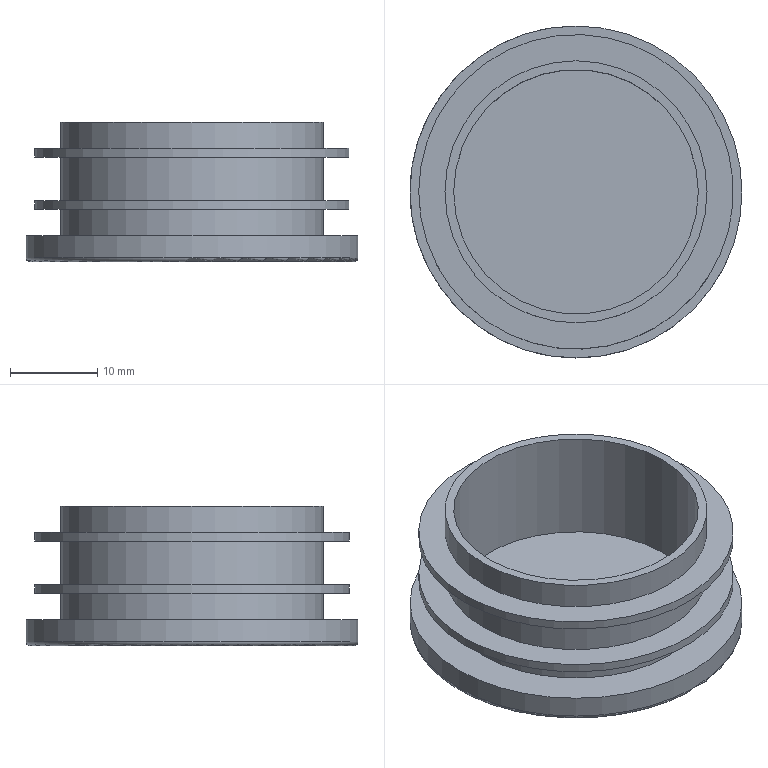Part | STEP file | 7101208W | 1 solid | 16 faces | box 38 x 38 x 16 mm | volume 5202 mm3 | plane 8 | cylinder 7 | torus 1 | commonest cylinder face diameters 30 x3 36 x2 28 x1 38 x1
STEP:
#1=CARTESIAN_POINT('',(0.,0.,0.));
#2=DIRECTION('',(0.,0.,1.));
#3=DIRECTION('',(1.,0.,0.));
#4=AXIS2_PLACEMENT_3D('',#1,#2,#3);
#5=CARTESIAN_POINT('',(15.,0.,3.));
#6=VERTEX_POINT('',#5);
#7=CARTESIAN_POINT('',(-15.,0.,3.));
#8=VERTEX_POINT('',#7);
#9=CARTESIAN_POINT('',(0.,0.,3.));
#10=DIRECTION('',(0.,0.,1.));
#11=DIRECTION('',(1.,0.,0.));
#12=AXIS2_PLACEMENT_3D('',#9,#10,#11);
#13=CIRCLE('',#12,15.);
#14=CARTESIAN_POINT('',(0.,0.,3.));
#15=DIRECTION('',(0.,0.,1.));
#16=DIRECTION('',(1.,0.,0.));
#17=AXIS2_PLACEMENT_3D('',#14,#15,#16);
#18=PLANE('',#17);
#19=CARTESIAN_POINT('',(0.,0.));
#20=DIRECTION('',(1.,0.));
#21=AXIS2_PLACEMENT_2D('',#19,#20);
#22=CIRCLE('',#21,15.);
#23=(GEOMETRIC_REPRESENTATION_CONTEXT(2)PARAMETRIC_REPRESENTATION_CONTEXT()REPRESENTATION_CONTEXT('',''));
#24=DEFINITIONAL_REPRESENTATION('',(#22),#23);
#25=PCURVE('',#18,#24);
#26=CARTESIAN_POINT('',(0.,0.,3.));
#27=DIRECTION('',(0.,0.,-1.));
#28=DIRECTION('',(-1.,0.,0.));
#29=AXIS2_PLACEMENT_3D('',#26,#27,#28);
#30=CYLINDRICAL_SURFACE('',#29,15.);
#31=CARTESIAN_POINT('',(3.142,0.));
#32=DIRECTION('',(-1.,0.));
#33=VECTOR('',#32,1.);
#34=LINE('',#31,#33);
#35=(GEOMETRIC_REPRESENTATION_CONTEXT(2)PARAMETRIC_REPRESENTATION_CONTEXT()REPRESENTATION_CONTEXT('',''));
#36=DEFINITIONAL_REPRESENTATION('',(#34),#35);
#37=PCURVE('',#30,#36);
#38=SURFACE_CURVE('',#13,(#25,#37),.PCURVE_S1.);
#39=EDGE_CURVE('',#6,#8,#38,.T.);
#40=ORIENTED_EDGE('',*,*,#39,.F.);
#41=CARTESIAN_POINT('',(0.,0.,3.));
#42=DIRECTION('',(0.,0.,1.));
#43=DIRECTION('',(1.,0.,0.));
#44=AXIS2_PLACEMENT_3D('',#41,#42,#43);
#45=CIRCLE('',#44,15.);
#46=CARTESIAN_POINT('',(0.,0.));
#47=DIRECTION('',(1.,0.));
#48=AXIS2_PLACEMENT_2D('',#46,#47);
#49=CIRCLE('',#48,15.);
#50=(GEOMETRIC_REPRESENTATION_CONTEXT(2)PARAMETRIC_REPRESENTATION_CONTEXT()REPRESENTATION_CONTEXT('',''));
#51=DEFINITIONAL_REPRESENTATION('',(#49),#50);
#52=PCURVE('',#18,#51);
#53=CARTESIAN_POINT('',(9.425,0.));
#54=DIRECTION('',(-1.,0.));
#55=VECTOR('',#54,1.);
#56=LINE('',#53,#55);
#57=(GEOMETRIC_REPRESENTATION_CONTEXT(2)PARAMETRIC_REPRESENTATION_CONTEXT()REPRESENTATION_CONTEXT('',''));
#58=DEFINITIONAL_REPRESENTATION('',(#56),#57);
#59=PCURVE('',#30,#58);
#60=SURFACE_CURVE('',#45,(#52,#59),.PCURVE_S1.);
#61=EDGE_CURVE('',#8,#6,#60,.T.);
#62=ORIENTED_EDGE('',*,*,#61,.F.);
#63=EDGE_LOOP('',(#40,#62));
#64=FACE_BOUND('',#63,.T.);
#65=CARTESIAN_POINT('',(19.,0.,3.));
#66=VERTEX_POINT('',#65);
#67=CARTESIAN_POINT('',(0.,0.,3.));
#68=DIRECTION('',(0.,0.,1.));
#69=DIRECTION('',(1.,0.,0.));
#70=AXIS2_PLACEMENT_3D('',#67,#68,#69);
#71=CIRCLE('',#70,19.);
#72=CARTESIAN_POINT('',(0.,0.));
#73=DIRECTION('',(1.,0.));
#74=AXIS2_PLACEMENT_2D('',#72,#73);
#75=CIRCLE('',#74,19.);
#76=(GEOMETRIC_REPRESENTATION_CONTEXT(2)PARAMETRIC_REPRESENTATION_CONTEXT()REPRESENTATION_CONTEXT('',''));
#77=DEFINITIONAL_REPRESENTATION('',(#75),#76);
#78=PCURVE('',#18,#77);
#79=CARTESIAN_POINT('',(0.,0.,3.));
#80=DIRECTION('',(0.,0.,-1.));
#81=DIRECTION('',(-1.,0.,0.));
#82=AXIS2_PLACEMENT_3D('',#79,#80,#81);
#83=CYLINDRICAL_SURFACE('',#82,19.);
#84=CARTESIAN_POINT('',(9.425,0.));
#85=DIRECTION('',(-1.,0.));
#86=VECTOR('',#85,1.);
#87=LINE('',#84,#86);
#88=(GEOMETRIC_REPRESENTATION_CONTEXT(2)PARAMETRIC_REPRESENTATION_CONTEXT()REPRESENTATION_CONTEXT('',''));
#89=DEFINITIONAL_REPRESENTATION('',(#87),#88);
#90=PCURVE('',#83,#89);
#91=SURFACE_CURVE('',#71,(#78,#90),.PCURVE_S1.);
#92=EDGE_CURVE('',#66,#66,#91,.T.);
#93=ORIENTED_EDGE('',*,*,#92,.T.);
#94=EDGE_LOOP('',(#93));
#95=FACE_BOUND('',#94,.T.);
#96=ADVANCED_FACE('',(#64,#95),#18,.T.);
#97=CARTESIAN_POINT('',(19.,0.,0.5));
#98=VERTEX_POINT('',#97);
#99=CARTESIAN_POINT('',(0.,0.,0.5));
#100=DIRECTION('',(0.,0.,1.));
#101=DIRECTION('',(1.,0.,0.));
#102=AXIS2_PLACEMENT_3D('',#99,#100,#101);
#103=CIRCLE('',#102,19.);
#104=CARTESIAN_POINT('',(9.425,2.5));
#105=DIRECTION('',(-1.,0.));
#106=VECTOR('',#105,1.);
#107=LINE('',#104,#106);
#108=(GEOMETRIC_REPRESENTATION_CONTEXT(2)PARAMETRIC_REPRESENTATION_CONTEXT()REPRESENTATION_CONTEXT('',''));
#109=DEFINITIONAL_REPRESENTATION('',(#107),#108);
#110=PCURVE('',#83,#109);
#111=CARTESIAN_POINT('',(0.,0.,0.5));
#112=DIRECTION('',(0.,0.,1.));
#113=DIRECTION('',(1.,0.,0.));
#114=AXIS2_PLACEMENT_3D('',#111,#112,#113);
#115=TOROIDAL_SURFACE('',#114,18.5,0.5);
#116=CARTESIAN_POINT('',(0.,6.283));
#117=DIRECTION('',(1.,0.));
#118=VECTOR('',#117,1.);
#119=LINE('',#116,#118);
#120=(GEOMETRIC_REPRESENTATION_CONTEXT(2)PARAMETRIC_REPRESENTATION_CONTEXT()REPRESENTATION_CONTEXT('',''));
#121=DEFINITIONAL_REPRESENTATION('',(#119),#120);
#122=PCURVE('',#115,#121);
#123=SURFACE_CURVE('',#103,(#110,#122),.PCURVE_S1.);
#124=EDGE_CURVE('',#98,#98,#123,.T.);
#125=ORIENTED_EDGE('',*,*,#124,.T.);
#126=CARTESIAN_POINT('',(19.,0.,3.));
#127=CARTESIAN_POINT('',(19.,0.,0.5));
#128=B_SPLINE_CURVE_WITH_KNOTS('',1,(#126,#127),.UNSPECIFIED.,.F.,.F.,(2,2),(0.,2.5),.PIECEWISE_BEZIER_KNOTS.);
#129=CARTESIAN_POINT('',(3.142,0.));
#130=DIRECTION('',(0.,1.));
#131=VECTOR('',#130,1.);
#132=LINE('',#129,#131);
#133=(GEOMETRIC_REPRESENTATION_CONTEXT(2)PARAMETRIC_REPRESENTATION_CONTEXT()REPRESENTATION_CONTEXT('',''));
#134=DEFINITIONAL_REPRESENTATION('',(#132),#133);
#135=PCURVE('',#83,#134);
#136=CARTESIAN_POINT('',(9.425,0.));
#137=DIRECTION('',(0.,1.));
#138=VECTOR('',#137,1.);
#139=LINE('',#136,#138);
#140=(GEOMETRIC_REPRESENTATION_CONTEXT(2)PARAMETRIC_REPRESENTATION_CONTEXT()REPRESENTATION_CONTEXT('',''));
#141=DEFINITIONAL_REPRESENTATION('',(#139),#140);
#142=PCURVE('',#83,#141);
#143=SEAM_CURVE('',#128,(#135,#142),.PCURVE_S1.);
#144=EDGE_CURVE('',#66,#98,#143,.T.);
#145=ORIENTED_EDGE('',*,*,#144,.F.);
#146=ORIENTED_EDGE('',*,*,#92,.F.);
#147=ORIENTED_EDGE('',*,*,#144,.T.);
#148=EDGE_LOOP('',(#125,#145,#146,#147));
#149=FACE_BOUND('',#148,.T.);
#150=ADVANCED_FACE('',(#149),#83,.T.);
#151=CARTESIAN_POINT('',(18.5,0.,0.));
#152=VERTEX_POINT('',#151);
#153=CARTESIAN_POINT('',(0.,0.,0.));
#154=DIRECTION('',(0.,0.,-1.));
#155=DIRECTION('',(1.,0.,0.));
#156=AXIS2_PLACEMENT_3D('',#153,#154,#155);
#157=CIRCLE('',#156,18.5);
#158=CARTESIAN_POINT('',(0.,0.,0.));
#159=DIRECTION('',(0.,0.,1.));
#160=DIRECTION('',(1.,0.,0.));
#161=AXIS2_PLACEMENT_3D('',#158,#159,#160);
#162=PLANE('',#161);
#163=CARTESIAN_POINT('',(18.5,0.));
#164=CARTESIAN_POINT('',(18.5,-32.043));
#165=CARTESIAN_POINT('',(-9.25,-16.021));
#166=CARTESIAN_POINT('',(-37.,0.));
#167=CARTESIAN_POINT('',(-9.25,16.021));
#168=CARTESIAN_POINT('',(18.5,32.043));
#169=CARTESIAN_POINT('',(18.5,0.));
#170=(BOUNDED_CURVE()B_SPLINE_CURVE(2,(#163,#164,#165,#166,#167,#168,#169),.UNSPECIFIED.,.T.,.F.)B_SPLINE_CURVE_WITH_KNOTS((1,2,2,2,2,1),(-2.094,0.,2.094,4.189,6.283,8.378),.UNSPECIFIED.)CURVE()GEOMETRIC_REPRESENTATION_ITEM()RATIONAL_B_SPLINE_CURVE((1.,0.5,1.,0.5,1.,0.5,1.))REPRESENTATION_ITEM(''));
#171=(GEOMETRIC_REPRESENTATION_CONTEXT(2)PARAMETRIC_REPRESENTATION_CONTEXT()REPRESENTATION_CONTEXT('',''));
#172=DEFINITIONAL_REPRESENTATION('',(#170),#171);
#173=PCURVE('',#162,#172);
#174=CARTESIAN_POINT('',(6.283,4.712));
#175=DIRECTION('',(-1.,0.));
#176=VECTOR('',#175,1.);
#177=LINE('',#174,#176);
#178=(GEOMETRIC_REPRESENTATION_CONTEXT(2)PARAMETRIC_REPRESENTATION_CONTEXT()REPRESENTATION_CONTEXT('',''));
#179=DEFINITIONAL_REPRESENTATION('',(#177),#178);
#180=PCURVE('',#115,#179);
#181=SURFACE_CURVE('',#157,(#173,#180),.PCURVE_S1.);
#182=EDGE_CURVE('',#152,#152,#181,.T.);
#183=ORIENTED_EDGE('',*,*,#182,.T.);
#184=EDGE_LOOP('',(#183));
#185=FACE_BOUND('',#184,.T.);
#186=ADVANCED_FACE('',(#185),#162,.F.);
#187=CARTESIAN_POINT('',(-15.,0.,6.));
#188=VERTEX_POINT('',#187);
#189=CARTESIAN_POINT('',(0.,0.,6.));
#190=DIRECTION('',(0.,0.,-1.));
#191=DIRECTION('',(-1.,0.,0.));
#192=AXIS2_PLACEMENT_3D('',#189,#190,#191);
#193=CIRCLE('',#192,15.);
#194=CARTESIAN_POINT('',(0.,-3.));
#195=DIRECTION('',(1.,0.));
#196=VECTOR('',#195,1.);
#197=LINE('',#194,#196);
#198=(GEOMETRIC_REPRESENTATION_CONTEXT(2)PARAMETRIC_REPRESENTATION_CONTEXT()REPRESENTATION_CONTEXT('',''));
#199=DEFINITIONAL_REPRESENTATION('',(#197),#198);
#200=PCURVE('',#30,#199);
#201=CARTESIAN_POINT('',(-15.,0.,6.));
#202=DIRECTION('',(0.,0.,-1.));
#203=DIRECTION('',(-1.,0.,0.));
#204=AXIS2_PLACEMENT_3D('',#201,#202,#203);
#205=PLANE('',#204);
#206=CARTESIAN_POINT('',(-15.,0.));
#207=DIRECTION('',(1.,0.));
#208=AXIS2_PLACEMENT_2D('',#206,#207);
#209=CIRCLE('',#208,15.);
#210=(GEOMETRIC_REPRESENTATION_CONTEXT(2)PARAMETRIC_REPRESENTATION_CONTEXT()REPRESENTATION_CONTEXT('',''));
#211=DEFINITIONAL_REPRESENTATION('',(#209),#210);
#212=PCURVE('',#205,#211);
#213=SURFACE_CURVE('',#193,(#200,#212),.PCURVE_S1.);
#214=EDGE_CURVE('',#188,#188,#213,.T.);
#215=ORIENTED_EDGE('',*,*,#214,.T.);
#216=CARTESIAN_POINT('',(-15.,0.,6.));
#217=CARTESIAN_POINT('',(-15.,0.,3.));
#218=B_SPLINE_CURVE_WITH_KNOTS('',1,(#216,#217),.UNSPECIFIED.,.F.,.F.,(2,2),(-3.,0.),.PIECEWISE_BEZIER_KNOTS.);
#219=CARTESIAN_POINT('',(6.283,0.));
#220=DIRECTION('',(0.,1.));
#221=VECTOR('',#220,1.);
#222=LINE('',#219,#221);
#223=(GEOMETRIC_REPRESENTATION_CONTEXT(2)PARAMETRIC_REPRESENTATION_CONTEXT()REPRESENTATION_CONTEXT('',''));
#224=DEFINITIONAL_REPRESENTATION('',(#222),#223);
#225=PCURVE('',#30,#224);
#226=CARTESIAN_POINT('',(0.,0.));
#227=DIRECTION('',(0.,1.));
#228=VECTOR('',#227,1.);
#229=LINE('',#226,#228);
#230=(GEOMETRIC_REPRESENTATION_CONTEXT(2)PARAMETRIC_REPRESENTATION_CONTEXT()REPRESENTATION_CONTEXT('',''));
#231=DEFINITIONAL_REPRESENTATION('',(#229),#230);
#232=PCURVE('',#30,#231);
#233=SEAM_CURVE('',#218,(#225,#232),.PCURVE_S1.);
#234=EDGE_CURVE('',#188,#8,#233,.T.);
#235=ORIENTED_EDGE('',*,*,#234,.T.);
#236=ORIENTED_EDGE('',*,*,#61,.T.);
#237=ORIENTED_EDGE('',*,*,#39,.T.);
#238=ORIENTED_EDGE('',*,*,#234,.F.);
#239=EDGE_LOOP('',(#215,#235,#236,#237,#238));
#240=FACE_BOUND('',#239,.T.);
#241=ADVANCED_FACE('',(#240),#30,.T.);
#242=CARTESIAN_POINT('',(-18.,0.,6.));
#243=VERTEX_POINT('',#242);
#244=CARTESIAN_POINT('',(0.,0.,6.));
#245=DIRECTION('',(0.,0.,-1.));
#246=DIRECTION('',(-1.,0.,0.));
#247=AXIS2_PLACEMENT_3D('',#244,#245,#246);
#248=CIRCLE('',#247,18.);
#249=CARTESIAN_POINT('',(-15.,0.));
#250=DIRECTION('',(1.,0.));
#251=AXIS2_PLACEMENT_2D('',#249,#250);
#252=CIRCLE('',#251,18.);
#253=(GEOMETRIC_REPRESENTATION_CONTEXT(2)PARAMETRIC_REPRESENTATION_CONTEXT()REPRESENTATION_CONTEXT('',''));
#254=DEFINITIONAL_REPRESENTATION('',(#252),#253);
#255=PCURVE('',#205,#254);
#256=CARTESIAN_POINT('',(0.,0.,3.));
#257=DIRECTION('',(0.,0.,-1.));
#258=DIRECTION('',(-1.,0.,0.));
#259=AXIS2_PLACEMENT_3D('',#256,#257,#258);
#260=CYLINDRICAL_SURFACE('',#259,18.);
#261=CARTESIAN_POINT('',(0.,-3.));
#262=DIRECTION('',(1.,0.));
#263=VECTOR('',#262,1.);
#264=LINE('',#261,#263);
#265=(GEOMETRIC_REPRESENTATION_CONTEXT(2)PARAMETRIC_REPRESENTATION_CONTEXT()REPRESENTATION_CONTEXT('',''));
#266=DEFINITIONAL_REPRESENTATION('',(#264),#265);
#267=PCURVE('',#260,#266);
#268=SURFACE_CURVE('',#248,(#255,#267),.PCURVE_S1.);
#269=EDGE_CURVE('',#243,#243,#268,.T.);
#270=ORIENTED_EDGE('',*,*,#269,.T.);
#271=EDGE_LOOP('',(#270));
#272=FACE_BOUND('',#271,.T.);
#273=ORIENTED_EDGE('',*,*,#214,.F.);
#274=EDGE_LOOP('',(#273));
#275=FACE_BOUND('',#274,.T.);
#276=ADVANCED_FACE('',(#272,#275),#205,.T.);
#277=CARTESIAN_POINT('',(-18.,0.,7.));
#278=VERTEX_POINT('',#277);
#279=CARTESIAN_POINT('',(0.,0.,7.));
#280=DIRECTION('',(0.,0.,-1.));
#281=DIRECTION('',(-1.,0.,0.));
#282=AXIS2_PLACEMENT_3D('',#279,#280,#281);
#283=CIRCLE('',#282,18.);
#284=CARTESIAN_POINT('',(0.,-4.));
#285=DIRECTION('',(1.,0.));
#286=VECTOR('',#285,1.);
#287=LINE('',#284,#286);
#288=(GEOMETRIC_REPRESENTATION_CONTEXT(2)PARAMETRIC_REPRESENTATION_CONTEXT()REPRESENTATION_CONTEXT('',''));
#289=DEFINITIONAL_REPRESENTATION('',(#287),#288);
#290=PCURVE('',#260,#289);
#291=CARTESIAN_POINT('',(-18.,0.,7.));
#292=DIRECTION('',(0.,0.,1.));
#293=DIRECTION('',(1.,0.,0.));
#294=AXIS2_PLACEMENT_3D('',#291,#292,#293);
#295=PLANE('',#294);
#296=CARTESIAN_POINT('',(0.,0.));
#297=CARTESIAN_POINT('',(0.,31.177));
#298=CARTESIAN_POINT('',(27.,15.588));
#299=CARTESIAN_POINT('',(54.,0.));
#300=CARTESIAN_POINT('',(27.,-15.588));
#301=CARTESIAN_POINT('',(0.,-31.177));
#302=CARTESIAN_POINT('',(0.,0.));
#303=(BOUNDED_CURVE()B_SPLINE_CURVE(2,(#296,#297,#298,#299,#300,#301,#302),.UNSPECIFIED.,.T.,.F.)B_SPLINE_CURVE_WITH_KNOTS((1,2,2,2,2,1),(-2.094,0.,2.094,4.189,6.283,8.378),.UNSPECIFIED.)CURVE()GEOMETRIC_REPRESENTATION_ITEM()RATIONAL_B_SPLINE_CURVE((1.,0.5,1.,0.5,1.,0.5,1.))REPRESENTATION_ITEM(''));
#304=(GEOMETRIC_REPRESENTATION_CONTEXT(2)PARAMETRIC_REPRESENTATION_CONTEXT()REPRESENTATION_CONTEXT('',''));
#305=DEFINITIONAL_REPRESENTATION('',(#303),#304);
#306=PCURVE('',#295,#305);
#307=SURFACE_CURVE('',#283,(#290,#306),.PCURVE_S1.);
#308=EDGE_CURVE('',#278,#278,#307,.T.);
#309=ORIENTED_EDGE('',*,*,#308,.T.);
#310=CARTESIAN_POINT('',(-18.,0.,7.));
#311=CARTESIAN_POINT('',(-18.,0.,6.));
#312=B_SPLINE_CURVE_WITH_KNOTS('',1,(#310,#311),.UNSPECIFIED.,.F.,.F.,(2,2),(-4.,-3.),.PIECEWISE_BEZIER_KNOTS.);
#313=CARTESIAN_POINT('',(6.283,0.));
#314=DIRECTION('',(0.,1.));
#315=VECTOR('',#314,1.);
#316=LINE('',#313,#315);
#317=(GEOMETRIC_REPRESENTATION_CONTEXT(2)PARAMETRIC_REPRESENTATION_CONTEXT()REPRESENTATION_CONTEXT('',''));
#318=DEFINITIONAL_REPRESENTATION('',(#316),#317);
#319=PCURVE('',#260,#318);
#320=CARTESIAN_POINT('',(0.,0.));
#321=DIRECTION('',(0.,1.));
#322=VECTOR('',#321,1.);
#323=LINE('',#320,#322);
#324=(GEOMETRIC_REPRESENTATION_CONTEXT(2)PARAMETRIC_REPRESENTATION_CONTEXT()REPRESENTATION_CONTEXT('',''));
#325=DEFINITIONAL_REPRESENTATION('',(#323),#324);
#326=PCURVE('',#260,#325);
#327=SEAM_CURVE('',#312,(#319,#326),.PCURVE_S1.);
#328=EDGE_CURVE('',#278,#243,#327,.T.);
#329=ORIENTED_EDGE('',*,*,#328,.T.);
#330=ORIENTED_EDGE('',*,*,#269,.F.);
#331=ORIENTED_EDGE('',*,*,#328,.F.);
#332=EDGE_LOOP('',(#309,#329,#330,#331));
#333=FACE_BOUND('',#332,.T.);
#334=ADVANCED_FACE('',(#333),#260,.T.);
#335=CARTESIAN_POINT('',(-15.,0.,7.));
#336=VERTEX_POINT('',#335);
#337=CARTESIAN_POINT('',(0.,0.,7.));
#338=DIRECTION('',(0.,0.,-1.));
#339=DIRECTION('',(-1.,0.,0.));
#340=AXIS2_PLACEMENT_3D('',#337,#338,#339);
#341=CIRCLE('',#340,15.);
#342=CARTESIAN_POINT('',(3.,0.));
#343=CARTESIAN_POINT('',(3.,25.981));
#344=CARTESIAN_POINT('',(25.5,12.99));
#345=CARTESIAN_POINT('',(48.,0.));
#346=CARTESIAN_POINT('',(25.5,-12.99));
#347=CARTESIAN_POINT('',(3.,-25.981));
#348=CARTESIAN_POINT('',(3.,0.));
#349=(BOUNDED_CURVE()B_SPLINE_CURVE(2,(#342,#343,#344,#345,#346,#347,#348),.UNSPECIFIED.,.T.,.F.)B_SPLINE_CURVE_WITH_KNOTS((1,2,2,2,2,1),(-2.094,0.,2.094,4.189,6.283,8.378),.UNSPECIFIED.)CURVE()GEOMETRIC_REPRESENTATION_ITEM()RATIONAL_B_SPLINE_CURVE((1.,0.5,1.,0.5,1.,0.5,1.))REPRESENTATION_ITEM(''));
#350=(GEOMETRIC_REPRESENTATION_CONTEXT(2)PARAMETRIC_REPRESENTATION_CONTEXT()REPRESENTATION_CONTEXT('',''));
#351=DEFINITIONAL_REPRESENTATION('',(#349),#350);
#352=PCURVE('',#295,#351);
#353=CARTESIAN_POINT('',(0.,0.,3.));
#354=DIRECTION('',(0.,0.,-1.));
#355=DIRECTION('',(-1.,0.,0.));
#356=AXIS2_PLACEMENT_3D('',#353,#354,#355);
#357=CYLINDRICAL_SURFACE('',#356,15.);
#358=CARTESIAN_POINT('',(0.,-4.));
#359=DIRECTION('',(1.,0.));
#360=VECTOR('',#359,1.);
#361=LINE('',#358,#360);
#362=(GEOMETRIC_REPRESENTATION_CONTEXT(2)PARAMETRIC_REPRESENTATION_CONTEXT()REPRESENTATION_CONTEXT('',''));
#363=DEFINITIONAL_REPRESENTATION('',(#361),#362);
#364=PCURVE('',#357,#363);
#365=SURFACE_CURVE('',#341,(#352,#364),.PCURVE_S1.);
#366=EDGE_CURVE('',#336,#336,#365,.T.);
#367=ORIENTED_EDGE('',*,*,#366,.T.);
#368=EDGE_LOOP('',(#367));
#369=FACE_BOUND('',#368,.T.);
#370=ORIENTED_EDGE('',*,*,#308,.F.);
#371=EDGE_LOOP('',(#370));
#372=FACE_BOUND('',#371,.T.);
#373=ADVANCED_FACE('',(#369,#372),#295,.T.);
#374=CARTESIAN_POINT('',(-15.,0.,12.));
#375=VERTEX_POINT('',#374);
#376=CARTESIAN_POINT('',(0.,0.,12.));
#377=DIRECTION('',(0.,0.,-1.));
#378=DIRECTION('',(-1.,0.,0.));
#379=AXIS2_PLACEMENT_3D('',#376,#377,#378);
#380=CIRCLE('',#379,15.);
#381=CARTESIAN_POINT('',(0.,-9.));
#382=DIRECTION('',(1.,0.));
#383=VECTOR('',#382,1.);
#384=LINE('',#381,#383);
#385=(GEOMETRIC_REPRESENTATION_CONTEXT(2)PARAMETRIC_REPRESENTATION_CONTEXT()REPRESENTATION_CONTEXT('',''));
#386=DEFINITIONAL_REPRESENTATION('',(#384),#385);
#387=PCURVE('',#357,#386);
#388=CARTESIAN_POINT('',(-15.,0.,12.));
#389=DIRECTION('',(0.,0.,-1.));
#390=DIRECTION('',(-1.,0.,0.));
#391=AXIS2_PLACEMENT_3D('',#388,#389,#390);
#392=PLANE('',#391);
#393=CARTESIAN_POINT('',(-15.,0.));
#394=DIRECTION('',(1.,0.));
#395=AXIS2_PLACEMENT_2D('',#393,#394);
#396=CIRCLE('',#395,15.);
#397=(GEOMETRIC_REPRESENTATION_CONTEXT(2)PARAMETRIC_REPRESENTATION_CONTEXT()REPRESENTATION_CONTEXT('',''));
#398=DEFINITIONAL_REPRESENTATION('',(#396),#397);
#399=PCURVE('',#392,#398);
#400=SURFACE_CURVE('',#380,(#387,#399),.PCURVE_S1.);
#401=EDGE_CURVE('',#375,#375,#400,.T.);
#402=ORIENTED_EDGE('',*,*,#401,.T.);
#403=CARTESIAN_POINT('',(-15.,0.,12.));
#404=CARTESIAN_POINT('',(-15.,0.,7.));
#405=B_SPLINE_CURVE_WITH_KNOTS('',1,(#403,#404),.UNSPECIFIED.,.F.,.F.,(2,2),(-9.,-4.),.PIECEWISE_BEZIER_KNOTS.);
#406=CARTESIAN_POINT('',(6.283,0.));
#407=DIRECTION('',(0.,1.));
#408=VECTOR('',#407,1.);
#409=LINE('',#406,#408);
#410=(GEOMETRIC_REPRESENTATION_CONTEXT(2)PARAMETRIC_REPRESENTATION_CONTEXT()REPRESENTATION_CONTEXT('',''));
#411=DEFINITIONAL_REPRESENTATION('',(#409),#410);
#412=PCURVE('',#357,#411);
#413=CARTESIAN_POINT('',(0.,0.));
#414=DIRECTION('',(0.,1.));
#415=VECTOR('',#414,1.);
#416=LINE('',#413,#415);
#417=(GEOMETRIC_REPRESENTATION_CONTEXT(2)PARAMETRIC_REPRESENTATION_CONTEXT()REPRESENTATION_CONTEXT('',''));
#418=DEFINITIONAL_REPRESENTATION('',(#416),#417);
#419=PCURVE('',#357,#418);
#420=SEAM_CURVE('',#405,(#412,#419),.PCURVE_S1.);
#421=EDGE_CURVE('',#375,#336,#420,.T.);
#422=ORIENTED_EDGE('',*,*,#421,.T.);
#423=ORIENTED_EDGE('',*,*,#366,.F.);
#424=ORIENTED_EDGE('',*,*,#421,.F.);
#425=EDGE_LOOP('',(#402,#422,#423,#424));
#426=FACE_BOUND('',#425,.T.);
#427=ADVANCED_FACE('',(#426),#357,.T.);
#428=CARTESIAN_POINT('',(-18.,0.,12.));
#429=VERTEX_POINT('',#428);
#430=CARTESIAN_POINT('',(0.,0.,12.));
#431=DIRECTION('',(0.,0.,-1.));
#432=DIRECTION('',(-1.,0.,0.));
#433=AXIS2_PLACEMENT_3D('',#430,#431,#432);
#434=CIRCLE('',#433,18.);
#435=CARTESIAN_POINT('',(-15.,0.));
#436=DIRECTION('',(1.,0.));
#437=AXIS2_PLACEMENT_2D('',#435,#436);
#438=CIRCLE('',#437,18.);
#439=(GEOMETRIC_REPRESENTATION_CONTEXT(2)PARAMETRIC_REPRESENTATION_CONTEXT()REPRESENTATION_CONTEXT('',''));
#440=DEFINITIONAL_REPRESENTATION('',(#438),#439);
#441=PCURVE('',#392,#440);
#442=CARTESIAN_POINT('',(0.,0.,3.));
#443=DIRECTION('',(0.,0.,-1.));
#444=DIRECTION('',(-1.,0.,0.));
#445=AXIS2_PLACEMENT_3D('',#442,#443,#444);
#446=CYLINDRICAL_SURFACE('',#445,18.);
#447=CARTESIAN_POINT('',(0.,-9.));
#448=DIRECTION('',(1.,0.));
#449=VECTOR('',#448,1.);
#450=LINE('',#447,#449);
#451=(GEOMETRIC_REPRESENTATION_CONTEXT(2)PARAMETRIC_REPRESENTATION_CONTEXT()REPRESENTATION_CONTEXT('',''));
#452=DEFINITIONAL_REPRESENTATION('',(#450),#451);
#453=PCURVE('',#446,#452);
#454=SURFACE_CURVE('',#434,(#441,#453),.PCURVE_S1.);
#455=EDGE_CURVE('',#429,#429,#454,.T.);
#456=ORIENTED_EDGE('',*,*,#455,.T.);
#457=EDGE_LOOP('',(#456));
#458=FACE_BOUND('',#457,.T.);
#459=ORIENTED_EDGE('',*,*,#401,.F.);
#460=EDGE_LOOP('',(#459));
#461=FACE_BOUND('',#460,.T.);
#462=ADVANCED_FACE('',(#458,#461),#392,.T.);
#463=CARTESIAN_POINT('',(-18.,0.,13.));
#464=VERTEX_POINT('',#463);
#465=CARTESIAN_POINT('',(0.,0.,13.));
#466=DIRECTION('',(0.,0.,-1.));
#467=DIRECTION('',(-1.,0.,0.));
#468=AXIS2_PLACEMENT_3D('',#465,#466,#467);
#469=CIRCLE('',#468,18.);
#470=CARTESIAN_POINT('',(0.,-10.));
#471=DIRECTION('',(1.,0.));
#472=VECTOR('',#471,1.);
#473=LINE('',#470,#472);
#474=(GEOMETRIC_REPRESENTATION_CONTEXT(2)PARAMETRIC_REPRESENTATION_CONTEXT()REPRESENTATION_CONTEXT('',''));
#475=DEFINITIONAL_REPRESENTATION('',(#473),#474);
#476=PCURVE('',#446,#475);
#477=CARTESIAN_POINT('',(-18.,0.,13.));
#478=DIRECTION('',(0.,0.,1.));
#479=DIRECTION('',(1.,0.,0.));
#480=AXIS2_PLACEMENT_3D('',#477,#478,#479);
#481=PLANE('',#480);
#482=CARTESIAN_POINT('',(0.,0.));
#483=CARTESIAN_POINT('',(0.,31.177));
#484=CARTESIAN_POINT('',(27.,15.588));
#485=CARTESIAN_POINT('',(54.,0.));
#486=CARTESIAN_POINT('',(27.,-15.588));
#487=CARTESIAN_POINT('',(0.,-31.177));
#488=CARTESIAN_POINT('',(0.,0.));
#489=(BOUNDED_CURVE()B_SPLINE_CURVE(2,(#482,#483,#484,#485,#486,#487,#488),.UNSPECIFIED.,.T.,.F.)B_SPLINE_CURVE_WITH_KNOTS((1,2,2,2,2,1),(-2.094,0.,2.094,4.189,6.283,8.378),.UNSPECIFIED.)CURVE()GEOMETRIC_REPRESENTATION_ITEM()RATIONAL_B_SPLINE_CURVE((1.,0.5,1.,0.5,1.,0.5,1.))REPRESENTATION_ITEM(''));
#490=(GEOMETRIC_REPRESENTATION_CONTEXT(2)PARAMETRIC_REPRESENTATION_CONTEXT()REPRESENTATION_CONTEXT('',''));
#491=DEFINITIONAL_REPRESENTATION('',(#489),#490);
#492=PCURVE('',#481,#491);
#493=SURFACE_CURVE('',#469,(#476,#492),.PCURVE_S1.);
#494=EDGE_CURVE('',#464,#464,#493,.T.);
#495=ORIENTED_EDGE('',*,*,#494,.T.);
#496=CARTESIAN_POINT('',(-18.,0.,13.));
#497=CARTESIAN_POINT('',(-18.,0.,12.));
#498=B_SPLINE_CURVE_WITH_KNOTS('',1,(#496,#497),.UNSPECIFIED.,.F.,.F.,(2,2),(-10.,-9.),.PIECEWISE_BEZIER_KNOTS.);
#499=CARTESIAN_POINT('',(6.283,0.));
#500=DIRECTION('',(0.,1.));
#501=VECTOR('',#500,1.);
#502=LINE('',#499,#501);
#503=(GEOMETRIC_REPRESENTATION_CONTEXT(2)PARAMETRIC_REPRESENTATION_CONTEXT()REPRESENTATION_CONTEXT('',''));
#504=DEFINITIONAL_REPRESENTATION('',(#502),#503);
#505=PCURVE('',#446,#504);
#506=CARTESIAN_POINT('',(0.,0.));
#507=DIRECTION('',(0.,1.));
#508=VECTOR('',#507,1.);
#509=LINE('',#506,#508);
#510=(GEOMETRIC_REPRESENTATION_CONTEXT(2)PARAMETRIC_REPRESENTATION_CONTEXT()REPRESENTATION_CONTEXT('',''));
#511=DEFINITIONAL_REPRESENTATION('',(#509),#510);
#512=PCURVE('',#446,#511);
#513=SEAM_CURVE('',#498,(#505,#512),.PCURVE_S1.);
#514=EDGE_CURVE('',#464,#429,#513,.T.);
#515=ORIENTED_EDGE('',*,*,#514,.T.);
#516=ORIENTED_EDGE('',*,*,#455,.F.);
#517=ORIENTED_EDGE('',*,*,#514,.F.);
#518=EDGE_LOOP('',(#495,#515,#516,#517));
#519=FACE_BOUND('',#518,.T.);
#520=ADVANCED_FACE('',(#519),#446,.T.);
#521=CARTESIAN_POINT('',(-15.,0.,13.));
#522=VERTEX_POINT('',#521);
#523=CARTESIAN_POINT('',(0.,0.,13.));
#524=DIRECTION('',(0.,0.,-1.));
#525=DIRECTION('',(-1.,0.,0.));
#526=AXIS2_PLACEMENT_3D('',#523,#524,#525);
#527=CIRCLE('',#526,15.);
#528=CARTESIAN_POINT('',(3.,0.));
#529=CARTESIAN_POINT('',(3.,25.981));
#530=CARTESIAN_POINT('',(25.5,12.99));
#531=CARTESIAN_POINT('',(48.,0.));
#532=CARTESIAN_POINT('',(25.5,-12.99));
#533=CARTESIAN_POINT('',(3.,-25.981));
#534=CARTESIAN_POINT('',(3.,0.));
#535=(BOUNDED_CURVE()B_SPLINE_CURVE(2,(#528,#529,#530,#531,#532,#533,#534),.UNSPECIFIED.,.T.,.F.)B_SPLINE_CURVE_WITH_KNOTS((1,2,2,2,2,1),(-2.094,0.,2.094,4.189,6.283,8.378),.UNSPECIFIED.)CURVE()GEOMETRIC_REPRESENTATION_ITEM()RATIONAL_B_SPLINE_CURVE((1.,0.5,1.,0.5,1.,0.5,1.))REPRESENTATION_ITEM(''));
#536=(GEOMETRIC_REPRESENTATION_CONTEXT(2)PARAMETRIC_REPRESENTATION_CONTEXT()REPRESENTATION_CONTEXT('',''));
#537=DEFINITIONAL_REPRESENTATION('',(#535),#536);
#538=PCURVE('',#481,#537);
#539=CARTESIAN_POINT('',(0.,0.,3.));
#540=DIRECTION('',(0.,0.,-1.));
#541=DIRECTION('',(-1.,0.,0.));
#542=AXIS2_PLACEMENT_3D('',#539,#540,#541);
#543=CYLINDRICAL_SURFACE('',#542,15.);
#544=CARTESIAN_POINT('',(0.,-10.));
#545=DIRECTION('',(1.,0.));
#546=VECTOR('',#545,1.);
#547=LINE('',#544,#546);
#548=(GEOMETRIC_REPRESENTATION_CONTEXT(2)PARAMETRIC_REPRESENTATION_CONTEXT()REPRESENTATION_CONTEXT('',''));
#549=DEFINITIONAL_REPRESENTATION('',(#547),#548);
#550=PCURVE('',#543,#549);
#551=SURFACE_CURVE('',#527,(#538,#550),.PCURVE_S1.);
#552=EDGE_CURVE('',#522,#522,#551,.T.);
#553=ORIENTED_EDGE('',*,*,#552,.T.);
#554=EDGE_LOOP('',(#553));
#555=FACE_BOUND('',#554,.T.);
#556=ORIENTED_EDGE('',*,*,#494,.F.);
#557=EDGE_LOOP('',(#556));
#558=FACE_BOUND('',#557,.T.);
#559=ADVANCED_FACE('',(#555,#558),#481,.T.);
#560=CARTESIAN_POINT('',(-15.,0.,16.));
#561=VERTEX_POINT('',#560);
#562=CARTESIAN_POINT('',(0.,0.,16.));
#563=DIRECTION('',(0.,0.,-1.));
#564=DIRECTION('',(-1.,0.,0.));
#565=AXIS2_PLACEMENT_3D('',#562,#563,#564);
#566=CIRCLE('',#565,15.);
#567=CARTESIAN_POINT('',(0.,-13.));
#568=DIRECTION('',(1.,0.));
#569=VECTOR('',#568,1.);
#570=LINE('',#567,#569);
#571=(GEOMETRIC_REPRESENTATION_CONTEXT(2)PARAMETRIC_REPRESENTATION_CONTEXT()REPRESENTATION_CONTEXT('',''));
#572=DEFINITIONAL_REPRESENTATION('',(#570),#571);
#573=PCURVE('',#543,#572);
#574=CARTESIAN_POINT('',(-15.,0.,16.));
#575=DIRECTION('',(0.,0.,1.));
#576=DIRECTION('',(1.,0.,0.));
#577=AXIS2_PLACEMENT_3D('',#574,#575,#576);
#578=PLANE('',#577);
#579=CARTESIAN_POINT('',(0.,0.));
#580=CARTESIAN_POINT('',(0.,25.981));
#581=CARTESIAN_POINT('',(22.5,12.99));
#582=CARTESIAN_POINT('',(45.,0.));
#583=CARTESIAN_POINT('',(22.5,-12.99));
#584=CARTESIAN_POINT('',(0.,-25.981));
#585=CARTESIAN_POINT('',(0.,0.));
#586=(BOUNDED_CURVE()B_SPLINE_CURVE(2,(#579,#580,#581,#582,#583,#584,#585),.UNSPECIFIED.,.T.,.F.)B_SPLINE_CURVE_WITH_KNOTS((1,2,2,2,2,1),(-2.094,0.,2.094,4.189,6.283,8.378),.UNSPECIFIED.)CURVE()GEOMETRIC_REPRESENTATION_ITEM()RATIONAL_B_SPLINE_CURVE((1.,0.5,1.,0.5,1.,0.5,1.))REPRESENTATION_ITEM(''));
#587=(GEOMETRIC_REPRESENTATION_CONTEXT(2)PARAMETRIC_REPRESENTATION_CONTEXT()REPRESENTATION_CONTEXT('',''));
#588=DEFINITIONAL_REPRESENTATION('',(#586),#587);
#589=PCURVE('',#578,#588);
#590=SURFACE_CURVE('',#566,(#573,#589),.PCURVE_S1.);
#591=EDGE_CURVE('',#561,#561,#590,.T.);
#592=ORIENTED_EDGE('',*,*,#591,.T.);
#593=CARTESIAN_POINT('',(-15.,0.,16.));
#594=CARTESIAN_POINT('',(-15.,0.,13.));
#595=B_SPLINE_CURVE_WITH_KNOTS('',1,(#593,#594),.UNSPECIFIED.,.F.,.F.,(2,2),(-13.,-10.),.PIECEWISE_BEZIER_KNOTS.);
#596=CARTESIAN_POINT('',(6.283,0.));
#597=DIRECTION('',(0.,1.));
#598=VECTOR('',#597,1.);
#599=LINE('',#596,#598);
#600=(GEOMETRIC_REPRESENTATION_CONTEXT(2)PARAMETRIC_REPRESENTATION_CONTEXT()REPRESENTATION_CONTEXT('',''));
#601=DEFINITIONAL_REPRESENTATION('',(#599),#600);
#602=PCURVE('',#543,#601);
#603=CARTESIAN_POINT('',(0.,0.));
#604=DIRECTION('',(0.,1.));
#605=VECTOR('',#604,1.);
#606=LINE('',#603,#605);
#607=(GEOMETRIC_REPRESENTATION_CONTEXT(2)PARAMETRIC_REPRESENTATION_CONTEXT()REPRESENTATION_CONTEXT('',''));
#608=DEFINITIONAL_REPRESENTATION('',(#606),#607);
#609=PCURVE('',#543,#608);
#610=SEAM_CURVE('',#595,(#602,#609),.PCURVE_S1.);
#611=EDGE_CURVE('',#561,#522,#610,.T.);
#612=ORIENTED_EDGE('',*,*,#611,.T.);
#613=ORIENTED_EDGE('',*,*,#552,.F.);
#614=ORIENTED_EDGE('',*,*,#611,.F.);
#615=EDGE_LOOP('',(#592,#612,#613,#614));
#616=FACE_BOUND('',#615,.T.);
#617=ADVANCED_FACE('',(#616),#543,.T.);
#618=CARTESIAN_POINT('',(-14.,0.,16.));
#619=VERTEX_POINT('',#618);
#620=CARTESIAN_POINT('',(0.,0.,16.));
#621=DIRECTION('',(0.,0.,-1.));
#622=DIRECTION('',(-1.,0.,0.));
#623=AXIS2_PLACEMENT_3D('',#620,#621,#622);
#624=CIRCLE('',#623,14.);
#625=CARTESIAN_POINT('',(1.,0.));
#626=CARTESIAN_POINT('',(1.,24.249));
#627=CARTESIAN_POINT('',(22.,12.124));
#628=CARTESIAN_POINT('',(43.,0.));
#629=CARTESIAN_POINT('',(22.,-12.124));
#630=CARTESIAN_POINT('',(1.,-24.249));
#631=CARTESIAN_POINT('',(1.,0.));
#632=(BOUNDED_CURVE()B_SPLINE_CURVE(2,(#625,#626,#627,#628,#629,#630,#631),.UNSPECIFIED.,.T.,.F.)B_SPLINE_CURVE_WITH_KNOTS((1,2,2,2,2,1),(-2.094,0.,2.094,4.189,6.283,8.378),.UNSPECIFIED.)CURVE()GEOMETRIC_REPRESENTATION_ITEM()RATIONAL_B_SPLINE_CURVE((1.,0.5,1.,0.5,1.,0.5,1.))REPRESENTATION_ITEM(''));
#633=(GEOMETRIC_REPRESENTATION_CONTEXT(2)PARAMETRIC_REPRESENTATION_CONTEXT()REPRESENTATION_CONTEXT('',''));
#634=DEFINITIONAL_REPRESENTATION('',(#632),#633);
#635=PCURVE('',#578,#634);
#636=CARTESIAN_POINT('',(0.,0.,3.));
#637=DIRECTION('',(0.,0.,-1.));
#638=DIRECTION('',(-1.,0.,0.));
#639=AXIS2_PLACEMENT_3D('',#636,#637,#638);
#640=CYLINDRICAL_SURFACE('',#639,14.);
#641=CARTESIAN_POINT('',(0.,-13.));
#642=DIRECTION('',(1.,0.));
#643=VECTOR('',#642,1.);
#644=LINE('',#641,#643);
#645=(GEOMETRIC_REPRESENTATION_CONTEXT(2)PARAMETRIC_REPRESENTATION_CONTEXT()REPRESENTATION_CONTEXT('',''));
#646=DEFINITIONAL_REPRESENTATION('',(#644),#645);
#647=PCURVE('',#640,#646);
#648=SURFACE_CURVE('',#624,(#635,#647),.PCURVE_S1.);
#649=EDGE_CURVE('',#619,#619,#648,.T.);
#650=ORIENTED_EDGE('',*,*,#649,.T.);
#651=EDGE_LOOP('',(#650));
#652=FACE_BOUND('',#651,.T.);
#653=ORIENTED_EDGE('',*,*,#591,.F.);
#654=EDGE_LOOP('',(#653));
#655=FACE_BOUND('',#654,.T.);
#656=ADVANCED_FACE('',(#652,#655),#578,.T.);
#657=CARTESIAN_POINT('',(-14.,0.,3.));
#658=VERTEX_POINT('',#657);
#659=CARTESIAN_POINT('',(14.,0.,3.));
#660=VERTEX_POINT('',#659);
#661=CARTESIAN_POINT('',(0.,0.,3.));
#662=DIRECTION('',(0.,0.,-1.));
#663=DIRECTION('',(1.,0.,0.));
#664=AXIS2_PLACEMENT_3D('',#661,#662,#663);
#665=CIRCLE('',#664,14.);
#666=CARTESIAN_POINT('',(-3.142,0.));
#667=DIRECTION('',(1.,0.));
#668=VECTOR('',#667,1.);
#669=LINE('',#666,#668);
#670=(GEOMETRIC_REPRESENTATION_CONTEXT(2)PARAMETRIC_REPRESENTATION_CONTEXT()REPRESENTATION_CONTEXT('',''));
#671=DEFINITIONAL_REPRESENTATION('',(#669),#670);
#672=PCURVE('',#640,#671);
#673=CARTESIAN_POINT('',(0.,0.,3.));
#674=DIRECTION('',(0.,0.,1.));
#675=DIRECTION('',(1.,0.,0.));
#676=AXIS2_PLACEMENT_3D('',#673,#674,#675);
#677=PLANE('',#676);
#678=CARTESIAN_POINT('',(14.,0.));
#679=CARTESIAN_POINT('',(14.,-24.249));
#680=CARTESIAN_POINT('',(-7.,-12.124));
#681=CARTESIAN_POINT('',(-28.,0.));
#682=CARTESIAN_POINT('',(-7.,12.124));
#683=CARTESIAN_POINT('',(14.,24.249));
#684=CARTESIAN_POINT('',(14.,0.));
#685=(BOUNDED_CURVE()B_SPLINE_CURVE(2,(#678,#679,#680,#681,#682,#683,#684),.UNSPECIFIED.,.T.,.F.)B_SPLINE_CURVE_WITH_KNOTS((1,2,2,2,2,1),(-2.094,0.,2.094,4.189,6.283,8.378),.UNSPECIFIED.)CURVE()GEOMETRIC_REPRESENTATION_ITEM()RATIONAL_B_SPLINE_CURVE((1.,0.5,1.,0.5,1.,0.5,1.))REPRESENTATION_ITEM(''));
#686=(GEOMETRIC_REPRESENTATION_CONTEXT(2)PARAMETRIC_REPRESENTATION_CONTEXT()REPRESENTATION_CONTEXT('',''));
#687=DEFINITIONAL_REPRESENTATION('',(#685),#686);
#688=PCURVE('',#677,#687);
#689=SURFACE_CURVE('',#665,(#672,#688),.PCURVE_S1.);
#690=EDGE_CURVE('',#658,#660,#689,.T.);
#691=ORIENTED_EDGE('',*,*,#690,.F.);
#692=CARTESIAN_POINT('',(-14.,0.,16.));
#693=CARTESIAN_POINT('',(-14.,0.,3.));
#694=B_SPLINE_CURVE_WITH_KNOTS('',1,(#692,#693),.UNSPECIFIED.,.F.,.F.,(2,2),(-13.,0.),.PIECEWISE_BEZIER_KNOTS.);
#695=CARTESIAN_POINT('',(0.,0.));
#696=DIRECTION('',(0.,1.));
#697=VECTOR('',#696,1.);
#698=LINE('',#695,#697);
#699=(GEOMETRIC_REPRESENTATION_CONTEXT(2)PARAMETRIC_REPRESENTATION_CONTEXT()REPRESENTATION_CONTEXT('',''));
#700=DEFINITIONAL_REPRESENTATION('',(#698),#699);
#701=PCURVE('',#640,#700);
#702=CARTESIAN_POINT('',(6.283,0.));
#703=DIRECTION('',(0.,1.));
#704=VECTOR('',#703,1.);
#705=LINE('',#702,#704);
#706=(GEOMETRIC_REPRESENTATION_CONTEXT(2)PARAMETRIC_REPRESENTATION_CONTEXT()REPRESENTATION_CONTEXT('',''));
#707=DEFINITIONAL_REPRESENTATION('',(#705),#706);
#708=PCURVE('',#640,#707);
#709=SEAM_CURVE('',#694,(#701,#708),.PCURVE_S1.);
#710=EDGE_CURVE('',#619,#658,#709,.T.);
#711=ORIENTED_EDGE('',*,*,#710,.F.);
#712=ORIENTED_EDGE('',*,*,#649,.T.);
#713=ORIENTED_EDGE('',*,*,#710,.T.);
#714=CARTESIAN_POINT('',(0.,0.,3.));
#715=DIRECTION('',(0.,0.,-1.));
#716=DIRECTION('',(1.,0.,0.));
#717=AXIS2_PLACEMENT_3D('',#714,#715,#716);
#718=CIRCLE('',#717,14.);
#719=CARTESIAN_POINT('',(3.142,0.));
#720=DIRECTION('',(1.,0.));
#721=VECTOR('',#720,1.);
#722=LINE('',#719,#721);
#723=(GEOMETRIC_REPRESENTATION_CONTEXT(2)PARAMETRIC_REPRESENTATION_CONTEXT()REPRESENTATION_CONTEXT('',''));
#724=DEFINITIONAL_REPRESENTATION('',(#722),#723);
#725=PCURVE('',#640,#724);
#726=CARTESIAN_POINT('',(14.,0.));
#727=CARTESIAN_POINT('',(14.,-24.249));
#728=CARTESIAN_POINT('',(-7.,-12.124));
#729=CARTESIAN_POINT('',(-28.,0.));
#730=CARTESIAN_POINT('',(-7.,12.124));
#731=CARTESIAN_POINT('',(14.,24.249));
#732=CARTESIAN_POINT('',(14.,0.));
#733=(BOUNDED_CURVE()B_SPLINE_CURVE(2,(#726,#727,#728,#729,#730,#731,#732),.UNSPECIFIED.,.T.,.F.)B_SPLINE_CURVE_WITH_KNOTS((1,2,2,2,2,1),(-2.094,0.,2.094,4.189,6.283,8.378),.UNSPECIFIED.)CURVE()GEOMETRIC_REPRESENTATION_ITEM()RATIONAL_B_SPLINE_CURVE((1.,0.5,1.,0.5,1.,0.5,1.))REPRESENTATION_ITEM(''));
#734=(GEOMETRIC_REPRESENTATION_CONTEXT(2)PARAMETRIC_REPRESENTATION_CONTEXT()REPRESENTATION_CONTEXT('',''));
#735=DEFINITIONAL_REPRESENTATION('',(#733),#734);
#736=PCURVE('',#677,#735);
#737=SURFACE_CURVE('',#718,(#725,#736),.PCURVE_S1.);
#738=EDGE_CURVE('',#660,#658,#737,.T.);
#739=ORIENTED_EDGE('',*,*,#738,.F.);
#740=EDGE_LOOP('',(#691,#711,#712,#713,#739));
#741=FACE_BOUND('',#740,.F.);
#742=ADVANCED_FACE('',(#741),#640,.F.);
#743=ORIENTED_EDGE('',*,*,#738,.F.);
#744=ORIENTED_EDGE('',*,*,#690,.F.);
#745=EDGE_LOOP('',(#743,#744));
#746=FACE_BOUND('',#745,.T.);
#747=ADVANCED_FACE('',(#746),#677,.T.);
#748=ORIENTED_EDGE('',*,*,#182,.F.);
#749=CARTESIAN_POINT('',(18.5,0.,0.));
#750=CARTESIAN_POINT('',(18.634,0.,0.));
#751=CARTESIAN_POINT('',(18.764,0.,0.0425));
#752=CARTESIAN_POINT('',(18.876,0.,0.124));
#753=CARTESIAN_POINT('',(18.957,0.,0.2361));
#754=CARTESIAN_POINT('',(19.,0.,0.3663));
#755=CARTESIAN_POINT('',(19.,0.,0.5));
#756=(BOUNDED_CURVE()B_SPLINE_CURVE(6,(#749,#750,#751,#752,#753,#754,#755),.UNSPECIFIED.,.F.,.F.)B_SPLINE_CURVE_WITH_KNOTS((7,7),(4.712,6.283),.PIECEWISE_BEZIER_KNOTS.)CURVE()GEOMETRIC_REPRESENTATION_ITEM()RATIONAL_B_SPLINE_CURVE((1.031,1.01,0.9979,0.994,0.9979,1.01,1.031))REPRESENTATION_ITEM(''));
#757=CARTESIAN_POINT('',(6.283,0.));
#758=DIRECTION('',(0.,1.));
#759=VECTOR('',#758,1.);
#760=LINE('',#757,#759);
#761=(GEOMETRIC_REPRESENTATION_CONTEXT(2)PARAMETRIC_REPRESENTATION_CONTEXT()REPRESENTATION_CONTEXT('',''));
#762=DEFINITIONAL_REPRESENTATION('',(#760),#761);
#763=PCURVE('',#115,#762);
#764=CARTESIAN_POINT('',(0.,0.));
#765=DIRECTION('',(0.,1.));
#766=VECTOR('',#765,1.);
#767=LINE('',#764,#766);
#768=(GEOMETRIC_REPRESENTATION_CONTEXT(2)PARAMETRIC_REPRESENTATION_CONTEXT()REPRESENTATION_CONTEXT('',''));
#769=DEFINITIONAL_REPRESENTATION('',(#767),#768);
#770=PCURVE('',#115,#769);
#771=SEAM_CURVE('',#756,(#763,#770),.PCURVE_S1.);
#772=EDGE_CURVE('',#152,#98,#771,.T.);
#773=ORIENTED_EDGE('',*,*,#772,.T.);
#774=ORIENTED_EDGE('',*,*,#124,.F.);
#775=ORIENTED_EDGE('',*,*,#772,.F.);
#776=EDGE_LOOP('',(#748,#773,#774,#775));
#777=FACE_BOUND('',#776,.T.);
#778=ADVANCED_FACE('',(#777),#115,.T.);
#779=CLOSED_SHELL('',(#96,#150,#186,#241,#276,#334,#373,#427,#462,#520,#559,#617,#656,#742,#747,#778));
#780=MANIFOLD_SOLID_BREP('',#779);
#781=(LENGTH_UNIT()NAMED_UNIT(*)SI_UNIT(.MILLI.,.METRE.));
#782=UNCERTAINTY_MEASURE_WITH_UNIT(LENGTH_MEASURE(0.000005),#781,'','');
#783=(NAMED_UNIT(*)PLANE_ANGLE_UNIT()SI_UNIT($,.RADIAN.));
#784=(NAMED_UNIT(*)SI_UNIT($,.STERADIAN.)SOLID_ANGLE_UNIT());
#785=(GEOMETRIC_REPRESENTATION_CONTEXT(3)GLOBAL_UNCERTAINTY_ASSIGNED_CONTEXT((#782))GLOBAL_UNIT_ASSIGNED_CONTEXT((#781,#783,#784))REPRESENTATION_CONTEXT('',''));
#786=ADVANCED_BREP_SHAPE_REPRESENTATION('',(#4,#780),#785);